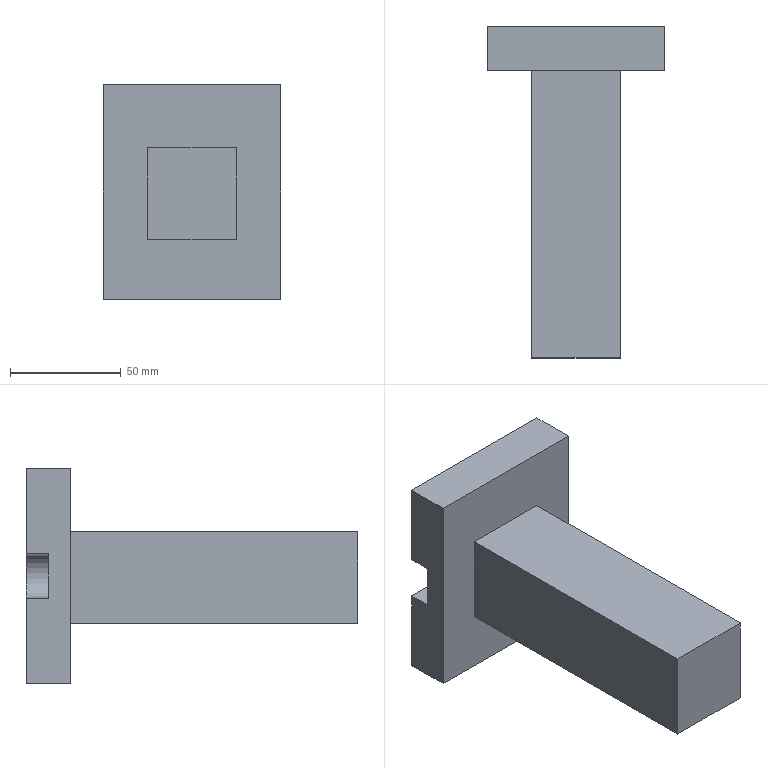Part | STEP file | Part1_4 | 1 solid | 15 faces | box 80 x 149.9 x 97 mm | volume 359263 mm3 | plane 14 | cylinder 1 | commonest cylinder face diameters 20 x1
STEP:
#1=CARTESIAN_POINT('',(0.,0.,0.));
#2=DIRECTION('',(0.,0.,1.));
#3=DIRECTION('',(1.,0.,0.));
#4=AXIS2_PLACEMENT_3D('',#1,#2,#3);
#5=CARTESIAN_POINT('',(10.,-29.9,-390.));
#6=VERTEX_POINT('',#5);
#7=CARTESIAN_POINT('',(-30.,-29.9,-390.));
#8=VERTEX_POINT('',#7);
#9=CARTESIAN_POINT('',(-30.,-29.9,-390.));
#10=DIRECTION('',(-1.,0.,0.));
#11=VECTOR('',#10,1.);
#12=LINE('',#9,#11);
#13=CARTESIAN_POINT('',(0.,-29.9,0.));
#14=DIRECTION('',(0.,1.,0.));
#15=DIRECTION('',(0.,0.,1.));
#16=AXIS2_PLACEMENT_3D('',#13,#14,#15);
#17=PLANE('',#16);
#18=CARTESIAN_POINT('',(-390.,-30.));
#19=DIRECTION('',(0.,-1.));
#20=VECTOR('',#19,1.);
#21=LINE('',#18,#20);
#22=(GEOMETRIC_REPRESENTATION_CONTEXT(2)PARAMETRIC_REPRESENTATION_CONTEXT()REPRESENTATION_CONTEXT('',''));
#23=DEFINITIONAL_REPRESENTATION('',(#21),#22);
#24=PCURVE('',#17,#23);
#25=CARTESIAN_POINT('',(-30.,100.,-390.));
#26=DIRECTION('',(0.,0.,-1.));
#27=DIRECTION('',(0.,1.,0.));
#28=AXIS2_PLACEMENT_3D('',#25,#26,#27);
#29=PLANE('',#28);
#30=CARTESIAN_POINT('',(-129.9,0.));
#31=DIRECTION('',(0.,-1.));
#32=VECTOR('',#31,1.);
#33=LINE('',#30,#32);
#34=(GEOMETRIC_REPRESENTATION_CONTEXT(2)PARAMETRIC_REPRESENTATION_CONTEXT()REPRESENTATION_CONTEXT('',''));
#35=DEFINITIONAL_REPRESENTATION('',(#33),#34);
#36=PCURVE('',#29,#35);
#37=SURFACE_CURVE('',#12,(#24,#36),.PCURVE_S1.);
#38=EDGE_CURVE('',#6,#8,#37,.T.);
#39=ORIENTED_EDGE('',*,*,#38,.T.);
#40=CARTESIAN_POINT('',(-30.,-29.9,-431.5));
#41=VERTEX_POINT('',#40);
#42=CARTESIAN_POINT('',(-30.,-29.9,-431.5));
#43=DIRECTION('',(0.,0.,-1.));
#44=VECTOR('',#43,1.);
#45=LINE('',#42,#44);
#46=CARTESIAN_POINT('',(-431.5,-30.));
#47=DIRECTION('',(-1.,0.));
#48=VECTOR('',#47,1.);
#49=LINE('',#46,#48);
#50=(GEOMETRIC_REPRESENTATION_CONTEXT(2)PARAMETRIC_REPRESENTATION_CONTEXT()REPRESENTATION_CONTEXT('',''));
#51=DEFINITIONAL_REPRESENTATION('',(#49),#50);
#52=PCURVE('',#17,#51);
#53=CARTESIAN_POINT('',(-30.,100.,-431.5));
#54=DIRECTION('',(1.,0.,0.));
#55=DIRECTION('',(0.,0.,-1.));
#56=AXIS2_PLACEMENT_3D('',#53,#54,#55);
#57=PLANE('',#56);
#58=CARTESIAN_POINT('',(0.,-129.9));
#59=DIRECTION('',(1.,0.));
#60=VECTOR('',#59,1.);
#61=LINE('',#58,#60);
#62=(GEOMETRIC_REPRESENTATION_CONTEXT(2)PARAMETRIC_REPRESENTATION_CONTEXT()REPRESENTATION_CONTEXT('',''));
#63=DEFINITIONAL_REPRESENTATION('',(#61),#62);
#64=PCURVE('',#57,#63);
#65=SURFACE_CURVE('',#45,(#52,#64),.PCURVE_S1.);
#66=EDGE_CURVE('',#8,#41,#65,.T.);
#67=ORIENTED_EDGE('',*,*,#66,.T.);
#68=CARTESIAN_POINT('',(10.,-29.9,-431.5));
#69=VERTEX_POINT('',#68);
#70=CARTESIAN_POINT('',(10.,-29.9,-431.5));
#71=DIRECTION('',(1.,0.,0.));
#72=VECTOR('',#71,1.);
#73=LINE('',#70,#72);
#74=CARTESIAN_POINT('',(-431.5,10.));
#75=DIRECTION('',(0.,1.));
#76=VECTOR('',#75,1.);
#77=LINE('',#74,#76);
#78=(GEOMETRIC_REPRESENTATION_CONTEXT(2)PARAMETRIC_REPRESENTATION_CONTEXT()REPRESENTATION_CONTEXT('',''));
#79=DEFINITIONAL_REPRESENTATION('',(#77),#78);
#80=PCURVE('',#17,#79);
#81=CARTESIAN_POINT('',(10.,100.,-431.5));
#82=DIRECTION('',(0.,0.,1.));
#83=DIRECTION('',(0.,-1.,0.));
#84=AXIS2_PLACEMENT_3D('',#81,#82,#83);
#85=PLANE('',#84);
#86=CARTESIAN_POINT('',(129.9,0.));
#87=DIRECTION('',(0.,1.));
#88=VECTOR('',#87,1.);
#89=LINE('',#86,#88);
#90=(GEOMETRIC_REPRESENTATION_CONTEXT(2)PARAMETRIC_REPRESENTATION_CONTEXT()REPRESENTATION_CONTEXT('',''));
#91=DEFINITIONAL_REPRESENTATION('',(#89),#90);
#92=PCURVE('',#85,#91);
#93=SURFACE_CURVE('',#73,(#80,#92),.PCURVE_S1.);
#94=EDGE_CURVE('',#41,#69,#93,.T.);
#95=ORIENTED_EDGE('',*,*,#94,.T.);
#96=CARTESIAN_POINT('',(10.,-29.9,-390.));
#97=DIRECTION('',(0.,0.,1.));
#98=VECTOR('',#97,1.);
#99=LINE('',#96,#98);
#100=CARTESIAN_POINT('',(-390.,10.));
#101=DIRECTION('',(1.,0.));
#102=VECTOR('',#101,1.);
#103=LINE('',#100,#102);
#104=(GEOMETRIC_REPRESENTATION_CONTEXT(2)PARAMETRIC_REPRESENTATION_CONTEXT()REPRESENTATION_CONTEXT('',''));
#105=DEFINITIONAL_REPRESENTATION('',(#103),#104);
#106=PCURVE('',#17,#105);
#107=CARTESIAN_POINT('',(10.,100.,-390.));
#108=DIRECTION('',(-1.,0.,0.));
#109=DIRECTION('',(0.,0.,1.));
#110=AXIS2_PLACEMENT_3D('',#107,#108,#109);
#111=PLANE('',#110);
#112=CARTESIAN_POINT('',(0.,-129.9));
#113=DIRECTION('',(1.,0.));
#114=VECTOR('',#113,1.);
#115=LINE('',#112,#114);
#116=(GEOMETRIC_REPRESENTATION_CONTEXT(2)PARAMETRIC_REPRESENTATION_CONTEXT()REPRESENTATION_CONTEXT('',''));
#117=DEFINITIONAL_REPRESENTATION('',(#115),#116);
#118=PCURVE('',#111,#117);
#119=SURFACE_CURVE('',#99,(#106,#118),.PCURVE_S1.);
#120=EDGE_CURVE('',#69,#6,#119,.T.);
#121=ORIENTED_EDGE('',*,*,#120,.T.);
#122=EDGE_LOOP('',(#39,#67,#95,#121));
#123=FACE_BOUND('',#122,.T.);
#124=ADVANCED_FACE('',(#123),#17,.F.);
#125=CARTESIAN_POINT('',(10.,100.,-431.5));
#126=VERTEX_POINT('',#125);
#127=CARTESIAN_POINT('',(10.,100.,-431.5));
#128=DIRECTION('',(0.,1.,0.));
#129=VECTOR('',#128,1.);
#130=LINE('',#127,#129);
#131=CARTESIAN_POINT('',(-41.5,0.));
#132=DIRECTION('',(0.,1.));
#133=VECTOR('',#132,1.);
#134=LINE('',#131,#133);
#135=(GEOMETRIC_REPRESENTATION_CONTEXT(2)PARAMETRIC_REPRESENTATION_CONTEXT()REPRESENTATION_CONTEXT('',''));
#136=DEFINITIONAL_REPRESENTATION('',(#134),#135);
#137=PCURVE('',#111,#136);
#138=CARTESIAN_POINT('',(0.,0.));
#139=DIRECTION('',(-1.,0.));
#140=VECTOR('',#139,1.);
#141=LINE('',#138,#140);
#142=(GEOMETRIC_REPRESENTATION_CONTEXT(2)PARAMETRIC_REPRESENTATION_CONTEXT()REPRESENTATION_CONTEXT('',''));
#143=DEFINITIONAL_REPRESENTATION('',(#141),#142);
#144=PCURVE('',#85,#143);
#145=SURFACE_CURVE('',#130,(#137,#144),.PCURVE_S1.);
#146=EDGE_CURVE('',#69,#126,#145,.T.);
#147=ORIENTED_EDGE('',*,*,#146,.T.);
#148=CARTESIAN_POINT('',(10.,100.,-390.));
#149=VERTEX_POINT('',#148);
#150=CARTESIAN_POINT('',(10.,100.,-361.5));
#151=DIRECTION('',(0.,0.,1.));
#152=VECTOR('',#151,1.);
#153=LINE('',#150,#152);
#154=CARTESIAN_POINT('',(28.5,0.));
#155=DIRECTION('',(1.,0.));
#156=VECTOR('',#155,1.);
#157=LINE('',#154,#156);
#158=(GEOMETRIC_REPRESENTATION_CONTEXT(2)PARAMETRIC_REPRESENTATION_CONTEXT()REPRESENTATION_CONTEXT('',''));
#159=DEFINITIONAL_REPRESENTATION('',(#157),#158);
#160=PCURVE('',#111,#159);
#161=CARTESIAN_POINT('',(-50.,100.,-361.5));
#162=DIRECTION('',(0.,1.,0.));
#163=DIRECTION('',(0.,0.,1.));
#164=AXIS2_PLACEMENT_3D('',#161,#162,#163);
#165=PLANE('',#164);
#166=CARTESIAN_POINT('',(0.,60.));
#167=DIRECTION('',(1.,0.));
#168=VECTOR('',#167,1.);
#169=LINE('',#166,#168);
#170=(GEOMETRIC_REPRESENTATION_CONTEXT(2)PARAMETRIC_REPRESENTATION_CONTEXT()REPRESENTATION_CONTEXT('',''));
#171=DEFINITIONAL_REPRESENTATION('',(#169),#170);
#172=PCURVE('',#165,#171);
#173=SURFACE_CURVE('',#153,(#160,#172),.PCURVE_S1.);
#174=EDGE_CURVE('',#126,#149,#173,.T.);
#175=ORIENTED_EDGE('',*,*,#174,.T.);
#176=CARTESIAN_POINT('',(10.,100.,-390.));
#177=DIRECTION('',(0.,-1.,0.));
#178=VECTOR('',#177,1.);
#179=LINE('',#176,#178);
#180=CARTESIAN_POINT('',(0.,0.));
#181=DIRECTION('',(0.,-1.));
#182=VECTOR('',#181,1.);
#183=LINE('',#180,#182);
#184=(GEOMETRIC_REPRESENTATION_CONTEXT(2)PARAMETRIC_REPRESENTATION_CONTEXT()REPRESENTATION_CONTEXT('',''));
#185=DEFINITIONAL_REPRESENTATION('',(#183),#184);
#186=PCURVE('',#111,#185);
#187=CARTESIAN_POINT('',(0.,40.));
#188=DIRECTION('',(-1.,0.));
#189=VECTOR('',#188,1.);
#190=LINE('',#187,#189);
#191=(GEOMETRIC_REPRESENTATION_CONTEXT(2)PARAMETRIC_REPRESENTATION_CONTEXT()REPRESENTATION_CONTEXT('',''));
#192=DEFINITIONAL_REPRESENTATION('',(#190),#191);
#193=PCURVE('',#29,#192);
#194=SURFACE_CURVE('',#179,(#186,#193),.PCURVE_S1.);
#195=EDGE_CURVE('',#149,#6,#194,.T.);
#196=ORIENTED_EDGE('',*,*,#195,.T.);
#197=ORIENTED_EDGE('',*,*,#120,.F.);
#198=EDGE_LOOP('',(#147,#175,#196,#197));
#199=FACE_BOUND('',#198,.T.);
#200=ADVANCED_FACE('',(#199),#111,.F.);
#201=ORIENTED_EDGE('',*,*,#195,.F.);
#202=CARTESIAN_POINT('',(-30.,100.,-390.));
#203=VERTEX_POINT('',#202);
#204=CARTESIAN_POINT('',(-50.,100.,-390.));
#205=DIRECTION('',(-1.,0.,0.));
#206=VECTOR('',#205,1.);
#207=LINE('',#204,#206);
#208=CARTESIAN_POINT('',(0.,-20.));
#209=DIRECTION('',(0.,-1.));
#210=VECTOR('',#209,1.);
#211=LINE('',#208,#210);
#212=(GEOMETRIC_REPRESENTATION_CONTEXT(2)PARAMETRIC_REPRESENTATION_CONTEXT()REPRESENTATION_CONTEXT('',''));
#213=DEFINITIONAL_REPRESENTATION('',(#211),#212);
#214=PCURVE('',#29,#213);
#215=CARTESIAN_POINT('',(-28.5,0.));
#216=DIRECTION('',(0.,-1.));
#217=VECTOR('',#216,1.);
#218=LINE('',#215,#217);
#219=(GEOMETRIC_REPRESENTATION_CONTEXT(2)PARAMETRIC_REPRESENTATION_CONTEXT()REPRESENTATION_CONTEXT('',''));
#220=DEFINITIONAL_REPRESENTATION('',(#218),#219);
#221=PCURVE('',#165,#220);
#222=SURFACE_CURVE('',#207,(#214,#221),.PCURVE_S1.);
#223=EDGE_CURVE('',#149,#203,#222,.T.);
#224=ORIENTED_EDGE('',*,*,#223,.T.);
#225=CARTESIAN_POINT('',(-30.,100.,-390.));
#226=DIRECTION('',(0.,-1.,0.));
#227=VECTOR('',#226,1.);
#228=LINE('',#225,#227);
#229=CARTESIAN_POINT('',(0.,0.));
#230=DIRECTION('',(-1.,0.));
#231=VECTOR('',#230,1.);
#232=LINE('',#229,#231);
#233=(GEOMETRIC_REPRESENTATION_CONTEXT(2)PARAMETRIC_REPRESENTATION_CONTEXT()REPRESENTATION_CONTEXT('',''));
#234=DEFINITIONAL_REPRESENTATION('',(#232),#233);
#235=PCURVE('',#29,#234);
#236=CARTESIAN_POINT('',(-41.5,0.));
#237=DIRECTION('',(0.,-1.));
#238=VECTOR('',#237,1.);
#239=LINE('',#236,#238);
#240=(GEOMETRIC_REPRESENTATION_CONTEXT(2)PARAMETRIC_REPRESENTATION_CONTEXT()REPRESENTATION_CONTEXT('',''));
#241=DEFINITIONAL_REPRESENTATION('',(#239),#240);
#242=PCURVE('',#57,#241);
#243=SURFACE_CURVE('',#228,(#235,#242),.PCURVE_S1.);
#244=EDGE_CURVE('',#203,#8,#243,.T.);
#245=ORIENTED_EDGE('',*,*,#244,.T.);
#246=ORIENTED_EDGE('',*,*,#38,.F.);
#247=EDGE_LOOP('',(#201,#224,#245,#246));
#248=FACE_BOUND('',#247,.T.);
#249=ADVANCED_FACE('',(#248),#29,.F.);
#250=ORIENTED_EDGE('',*,*,#244,.F.);
#251=CARTESIAN_POINT('',(-30.,100.,-431.5));
#252=VERTEX_POINT('',#251);
#253=CARTESIAN_POINT('',(-30.,100.,-361.5));
#254=DIRECTION('',(0.,0.,-1.));
#255=VECTOR('',#254,1.);
#256=LINE('',#253,#255);
#257=CARTESIAN_POINT('',(-70.,0.));
#258=DIRECTION('',(1.,0.));
#259=VECTOR('',#258,1.);
#260=LINE('',#257,#259);
#261=(GEOMETRIC_REPRESENTATION_CONTEXT(2)PARAMETRIC_REPRESENTATION_CONTEXT()REPRESENTATION_CONTEXT('',''));
#262=DEFINITIONAL_REPRESENTATION('',(#260),#261);
#263=PCURVE('',#57,#262);
#264=CARTESIAN_POINT('',(0.,20.));
#265=DIRECTION('',(-1.,0.));
#266=VECTOR('',#265,1.);
#267=LINE('',#264,#266);
#268=(GEOMETRIC_REPRESENTATION_CONTEXT(2)PARAMETRIC_REPRESENTATION_CONTEXT()REPRESENTATION_CONTEXT('',''));
#269=DEFINITIONAL_REPRESENTATION('',(#267),#268);
#270=PCURVE('',#165,#269);
#271=SURFACE_CURVE('',#256,(#263,#270),.PCURVE_S1.);
#272=EDGE_CURVE('',#203,#252,#271,.T.);
#273=ORIENTED_EDGE('',*,*,#272,.T.);
#274=CARTESIAN_POINT('',(-30.,100.,-431.5));
#275=DIRECTION('',(0.,-1.,0.));
#276=VECTOR('',#275,1.);
#277=LINE('',#274,#276);
#278=CARTESIAN_POINT('',(0.,0.));
#279=DIRECTION('',(0.,-1.));
#280=VECTOR('',#279,1.);
#281=LINE('',#278,#280);
#282=(GEOMETRIC_REPRESENTATION_CONTEXT(2)PARAMETRIC_REPRESENTATION_CONTEXT()REPRESENTATION_CONTEXT('',''));
#283=DEFINITIONAL_REPRESENTATION('',(#281),#282);
#284=PCURVE('',#57,#283);
#285=CARTESIAN_POINT('',(0.,-40.));
#286=DIRECTION('',(1.,0.));
#287=VECTOR('',#286,1.);
#288=LINE('',#285,#287);
#289=(GEOMETRIC_REPRESENTATION_CONTEXT(2)PARAMETRIC_REPRESENTATION_CONTEXT()REPRESENTATION_CONTEXT('',''));
#290=DEFINITIONAL_REPRESENTATION('',(#288),#289);
#291=PCURVE('',#85,#290);
#292=SURFACE_CURVE('',#277,(#284,#291),.PCURVE_S1.);
#293=EDGE_CURVE('',#252,#41,#292,.T.);
#294=ORIENTED_EDGE('',*,*,#293,.T.);
#295=ORIENTED_EDGE('',*,*,#66,.F.);
#296=EDGE_LOOP('',(#250,#273,#294,#295));
#297=FACE_BOUND('',#296,.T.);
#298=ADVANCED_FACE('',(#297),#57,.F.);
#299=ORIENTED_EDGE('',*,*,#293,.F.);
#300=CARTESIAN_POINT('',(-50.,100.,-431.5));
#301=DIRECTION('',(1.,0.,0.));
#302=VECTOR('',#301,1.);
#303=LINE('',#300,#302);
#304=CARTESIAN_POINT('',(0.,-60.));
#305=DIRECTION('',(0.,1.));
#306=VECTOR('',#305,1.);
#307=LINE('',#304,#306);
#308=(GEOMETRIC_REPRESENTATION_CONTEXT(2)PARAMETRIC_REPRESENTATION_CONTEXT()REPRESENTATION_CONTEXT('',''));
#309=DEFINITIONAL_REPRESENTATION('',(#307),#308);
#310=PCURVE('',#85,#309);
#311=CARTESIAN_POINT('',(-70.,0.));
#312=DIRECTION('',(0.,1.));
#313=VECTOR('',#312,1.);
#314=LINE('',#311,#313);
#315=(GEOMETRIC_REPRESENTATION_CONTEXT(2)PARAMETRIC_REPRESENTATION_CONTEXT()REPRESENTATION_CONTEXT('',''));
#316=DEFINITIONAL_REPRESENTATION('',(#314),#315);
#317=PCURVE('',#165,#316);
#318=SURFACE_CURVE('',#303,(#310,#317),.PCURVE_S1.);
#319=EDGE_CURVE('',#252,#126,#318,.T.);
#320=ORIENTED_EDGE('',*,*,#319,.T.);
#321=ORIENTED_EDGE('',*,*,#146,.F.);
#322=ORIENTED_EDGE('',*,*,#94,.F.);
#323=EDGE_LOOP('',(#299,#320,#321,#322));
#324=FACE_BOUND('',#323,.T.);
#325=ADVANCED_FACE('',(#324),#85,.F.);
#326=ORIENTED_EDGE('',*,*,#272,.F.);
#327=ORIENTED_EDGE('',*,*,#223,.F.);
#328=ORIENTED_EDGE('',*,*,#174,.F.);
#329=ORIENTED_EDGE('',*,*,#319,.F.);
#330=EDGE_LOOP('',(#326,#327,#328,#329));
#331=FACE_BOUND('',#330,.T.);
#332=CARTESIAN_POINT('',(30.,100.,-361.5));
#333=VERTEX_POINT('',#332);
#334=CARTESIAN_POINT('',(30.,100.,-458.5));
#335=VERTEX_POINT('',#334);
#336=CARTESIAN_POINT('',(30.,100.,-361.5));
#337=DIRECTION('',(0.,0.,-1.));
#338=VECTOR('',#337,1.);
#339=LINE('',#336,#338);
#340=CARTESIAN_POINT('',(0.,80.));
#341=DIRECTION('',(-1.,0.));
#342=VECTOR('',#341,1.);
#343=LINE('',#340,#342);
#344=(GEOMETRIC_REPRESENTATION_CONTEXT(2)PARAMETRIC_REPRESENTATION_CONTEXT()REPRESENTATION_CONTEXT('',''));
#345=DEFINITIONAL_REPRESENTATION('',(#343),#344);
#346=PCURVE('',#165,#345);
#347=CARTESIAN_POINT('',(30.,120.,-361.5));
#348=DIRECTION('',(1.,0.,0.));
#349=DIRECTION('',(0.,0.,-1.));
#350=AXIS2_PLACEMENT_3D('',#347,#348,#349);
#351=PLANE('',#350);
#352=CARTESIAN_POINT('',(0.,-20.));
#353=DIRECTION('',(1.,0.));
#354=VECTOR('',#353,1.);
#355=LINE('',#352,#354);
#356=(GEOMETRIC_REPRESENTATION_CONTEXT(2)PARAMETRIC_REPRESENTATION_CONTEXT()REPRESENTATION_CONTEXT('',''));
#357=DEFINITIONAL_REPRESENTATION('',(#355),#356);
#358=PCURVE('',#351,#357);
#359=SURFACE_CURVE('',#339,(#346,#358),.PCURVE_S1.);
#360=EDGE_CURVE('',#333,#335,#359,.T.);
#361=ORIENTED_EDGE('',*,*,#360,.F.);
#362=CARTESIAN_POINT('',(-50.,100.,-361.5));
#363=VERTEX_POINT('',#362);
#364=CARTESIAN_POINT('',(0.,100.,-361.5));
#365=DIRECTION('',(1.,0.,0.));
#366=VECTOR('',#365,1.);
#367=LINE('',#364,#366);
#368=CARTESIAN_POINT('',(0.,50.));
#369=DIRECTION('',(0.,1.));
#370=VECTOR('',#369,1.);
#371=LINE('',#368,#370);
#372=(GEOMETRIC_REPRESENTATION_CONTEXT(2)PARAMETRIC_REPRESENTATION_CONTEXT()REPRESENTATION_CONTEXT('',''));
#373=DEFINITIONAL_REPRESENTATION('',(#371),#372);
#374=PCURVE('',#165,#373);
#375=CARTESIAN_POINT('',(0.,0.,-361.5));
#376=DIRECTION('',(0.,0.,1.));
#377=DIRECTION('',(1.,0.,0.));
#378=AXIS2_PLACEMENT_3D('',#375,#376,#377);
#379=PLANE('',#378);
#380=CARTESIAN_POINT('',(0.,100.));
#381=DIRECTION('',(1.,0.));
#382=VECTOR('',#381,1.);
#383=LINE('',#380,#382);
#384=(GEOMETRIC_REPRESENTATION_CONTEXT(2)PARAMETRIC_REPRESENTATION_CONTEXT()REPRESENTATION_CONTEXT('',''));
#385=DEFINITIONAL_REPRESENTATION('',(#383),#384);
#386=PCURVE('',#379,#385);
#387=SURFACE_CURVE('',#367,(#374,#386),.PCURVE_S1.);
#388=EDGE_CURVE('',#363,#333,#387,.T.);
#389=ORIENTED_EDGE('',*,*,#388,.F.);
#390=CARTESIAN_POINT('',(-50.,100.,-458.5));
#391=VERTEX_POINT('',#390);
#392=CARTESIAN_POINT('',(-50.,100.,-361.5));
#393=DIRECTION('',(0.,0.,1.));
#394=VECTOR('',#393,1.);
#395=LINE('',#392,#394);
#396=CARTESIAN_POINT('',(0.,0.));
#397=DIRECTION('',(1.,0.));
#398=VECTOR('',#397,1.);
#399=LINE('',#396,#398);
#400=(GEOMETRIC_REPRESENTATION_CONTEXT(2)PARAMETRIC_REPRESENTATION_CONTEXT()REPRESENTATION_CONTEXT('',''));
#401=DEFINITIONAL_REPRESENTATION('',(#399),#400);
#402=PCURVE('',#165,#401);
#403=CARTESIAN_POINT('',(-50.,100.,-361.5));
#404=DIRECTION('',(-1.,0.,0.));
#405=DIRECTION('',(0.,0.,1.));
#406=AXIS2_PLACEMENT_3D('',#403,#404,#405);
#407=PLANE('',#406);
#408=CARTESIAN_POINT('',(0.,0.));
#409=DIRECTION('',(1.,0.));
#410=VECTOR('',#409,1.);
#411=LINE('',#408,#410);
#412=(GEOMETRIC_REPRESENTATION_CONTEXT(2)PARAMETRIC_REPRESENTATION_CONTEXT()REPRESENTATION_CONTEXT('',''));
#413=DEFINITIONAL_REPRESENTATION('',(#411),#412);
#414=PCURVE('',#407,#413);
#415=SURFACE_CURVE('',#395,(#402,#414),.PCURVE_S1.);
#416=EDGE_CURVE('',#391,#363,#415,.T.);
#417=ORIENTED_EDGE('',*,*,#416,.F.);
#418=CARTESIAN_POINT('',(-25.,100.,-458.5));
#419=DIRECTION('',(-1.,0.,0.));
#420=VECTOR('',#419,1.);
#421=LINE('',#418,#420);
#422=CARTESIAN_POINT('',(-97.,25.));
#423=DIRECTION('',(0.,-1.));
#424=VECTOR('',#423,1.);
#425=LINE('',#422,#424);
#426=(GEOMETRIC_REPRESENTATION_CONTEXT(2)PARAMETRIC_REPRESENTATION_CONTEXT()REPRESENTATION_CONTEXT('',''));
#427=DEFINITIONAL_REPRESENTATION('',(#425),#426);
#428=PCURVE('',#165,#427);
#429=CARTESIAN_POINT('',(-25.,377.,-458.5));
#430=DIRECTION('',(0.,0.,-1.));
#431=DIRECTION('',(-1.,0.,0.));
#432=AXIS2_PLACEMENT_3D('',#429,#430,#431);
#433=PLANE('',#432);
#434=CARTESIAN_POINT('',(0.,-277.));
#435=DIRECTION('',(1.,0.));
#436=VECTOR('',#435,1.);
#437=LINE('',#434,#436);
#438=(GEOMETRIC_REPRESENTATION_CONTEXT(2)PARAMETRIC_REPRESENTATION_CONTEXT()REPRESENTATION_CONTEXT('',''));
#439=DEFINITIONAL_REPRESENTATION('',(#437),#438);
#440=PCURVE('',#433,#439);
#441=SURFACE_CURVE('',#421,(#428,#440),.PCURVE_S1.);
#442=EDGE_CURVE('',#335,#391,#441,.T.);
#443=ORIENTED_EDGE('',*,*,#442,.F.);
#444=EDGE_LOOP('',(#361,#389,#417,#443));
#445=FACE_BOUND('',#444,.T.);
#446=ADVANCED_FACE('',(#331,#445),#165,.F.);
#447=CARTESIAN_POINT('',(0.,110.,-420.));
#448=VERTEX_POINT('',#447);
#449=CARTESIAN_POINT('',(-50.,110.,-420.));
#450=VERTEX_POINT('',#449);
#451=CARTESIAN_POINT('',(-60.,110.,-420.));
#452=DIRECTION('',(-1.,0.,0.));
#453=VECTOR('',#452,1.);
#454=LINE('',#451,#453);
#455=CARTESIAN_POINT('',(0.,110.,0.));
#456=DIRECTION('',(0.,1.,0.));
#457=DIRECTION('',(0.,0.,1.));
#458=AXIS2_PLACEMENT_3D('',#455,#456,#457);
#459=PLANE('',#458);
#460=CARTESIAN_POINT('',(-420.,-60.));
#461=DIRECTION('',(0.,-1.));
#462=VECTOR('',#461,1.);
#463=LINE('',#460,#462);
#464=(GEOMETRIC_REPRESENTATION_CONTEXT(2)PARAMETRIC_REPRESENTATION_CONTEXT()REPRESENTATION_CONTEXT('',''));
#465=DEFINITIONAL_REPRESENTATION('',(#463),#464);
#466=PCURVE('',#459,#465);
#467=CARTESIAN_POINT('',(-60.,120.,-420.));
#468=DIRECTION('',(0.,0.,-1.));
#469=DIRECTION('',(0.,1.,0.));
#470=AXIS2_PLACEMENT_3D('',#467,#468,#469);
#471=PLANE('',#470);
#472=CARTESIAN_POINT('',(-10.,0.));
#473=DIRECTION('',(0.,-1.));
#474=VECTOR('',#473,1.);
#475=LINE('',#472,#474);
#476=(GEOMETRIC_REPRESENTATION_CONTEXT(2)PARAMETRIC_REPRESENTATION_CONTEXT()REPRESENTATION_CONTEXT('',''));
#477=DEFINITIONAL_REPRESENTATION('',(#475),#476);
#478=PCURVE('',#471,#477);
#479=SURFACE_CURVE('',#454,(#466,#478),.PCURVE_S1.);
#480=EDGE_CURVE('',#448,#450,#479,.T.);
#481=ORIENTED_EDGE('',*,*,#480,.T.);
#482=CARTESIAN_POINT('',(-50.,110.,-400.));
#483=VERTEX_POINT('',#482);
#484=CARTESIAN_POINT('',(-50.,110.,-361.5));
#485=DIRECTION('',(0.,0.,-1.));
#486=VECTOR('',#485,1.);
#487=LINE('',#484,#486);
#488=CARTESIAN_POINT('',(-361.5,-50.));
#489=DIRECTION('',(-1.,0.));
#490=VECTOR('',#489,1.);
#491=LINE('',#488,#490);
#492=(GEOMETRIC_REPRESENTATION_CONTEXT(2)PARAMETRIC_REPRESENTATION_CONTEXT()REPRESENTATION_CONTEXT('',''));
#493=DEFINITIONAL_REPRESENTATION('',(#491),#492);
#494=PCURVE('',#459,#493);
#495=CARTESIAN_POINT('',(0.,10.));
#496=DIRECTION('',(-1.,0.));
#497=VECTOR('',#496,1.);
#498=LINE('',#495,#497);
#499=(GEOMETRIC_REPRESENTATION_CONTEXT(2)PARAMETRIC_REPRESENTATION_CONTEXT()REPRESENTATION_CONTEXT('',''));
#500=DEFINITIONAL_REPRESENTATION('',(#498),#499);
#501=PCURVE('',#407,#500);
#502=SURFACE_CURVE('',#487,(#494,#501),.PCURVE_S1.);
#503=EDGE_CURVE('',#483,#450,#502,.T.);
#504=ORIENTED_EDGE('',*,*,#503,.F.);
#505=CARTESIAN_POINT('',(0.,110.,-400.));
#506=VERTEX_POINT('',#505);
#507=CARTESIAN_POINT('',(0.,110.,-400.));
#508=DIRECTION('',(1.,0.,0.));
#509=VECTOR('',#508,1.);
#510=LINE('',#507,#509);
#511=CARTESIAN_POINT('',(-400.,0.));
#512=DIRECTION('',(0.,1.));
#513=VECTOR('',#512,1.);
#514=LINE('',#511,#513);
#515=(GEOMETRIC_REPRESENTATION_CONTEXT(2)PARAMETRIC_REPRESENTATION_CONTEXT()REPRESENTATION_CONTEXT('',''));
#516=DEFINITIONAL_REPRESENTATION('',(#514),#515);
#517=PCURVE('',#459,#516);
#518=CARTESIAN_POINT('',(0.,120.,-400.));
#519=DIRECTION('',(0.,0.,1.));
#520=DIRECTION('',(0.,-1.,0.));
#521=AXIS2_PLACEMENT_3D('',#518,#519,#520);
#522=PLANE('',#521);
#523=CARTESIAN_POINT('',(10.,0.));
#524=DIRECTION('',(0.,1.));
#525=VECTOR('',#524,1.);
#526=LINE('',#523,#525);
#527=(GEOMETRIC_REPRESENTATION_CONTEXT(2)PARAMETRIC_REPRESENTATION_CONTEXT()REPRESENTATION_CONTEXT('',''));
#528=DEFINITIONAL_REPRESENTATION('',(#526),#527);
#529=PCURVE('',#522,#528);
#530=SURFACE_CURVE('',#510,(#517,#529),.PCURVE_S1.);
#531=EDGE_CURVE('',#483,#506,#530,.T.);
#532=ORIENTED_EDGE('',*,*,#531,.T.);
#533=CARTESIAN_POINT('',(0.,110.,-410.));
#534=DIRECTION('',(0.,1.,0.));
#535=DIRECTION('',(0.,0.,1.));
#536=AXIS2_PLACEMENT_3D('',#533,#534,#535);
#537=CIRCLE('',#536,10.);
#538=CARTESIAN_POINT('',(-410.,0.));
#539=DIRECTION('',(1.,0.));
#540=AXIS2_PLACEMENT_2D('',#538,#539);
#541=CIRCLE('',#540,10.);
#542=(GEOMETRIC_REPRESENTATION_CONTEXT(2)PARAMETRIC_REPRESENTATION_CONTEXT()REPRESENTATION_CONTEXT('',''));
#543=DEFINITIONAL_REPRESENTATION('',(#541),#542);
#544=PCURVE('',#459,#543);
#545=CARTESIAN_POINT('',(0.,115.,-410.));
#546=DIRECTION('',(0.,1.,0.));
#547=DIRECTION('',(0.,0.,1.));
#548=AXIS2_PLACEMENT_3D('',#545,#546,#547);
#549=CYLINDRICAL_SURFACE('',#548,10.);
#550=CARTESIAN_POINT('',(0.,-5.));
#551=DIRECTION('',(1.,0.));
#552=VECTOR('',#551,1.);
#553=LINE('',#550,#552);
#554=(GEOMETRIC_REPRESENTATION_CONTEXT(2)PARAMETRIC_REPRESENTATION_CONTEXT()REPRESENTATION_CONTEXT('',''));
#555=DEFINITIONAL_REPRESENTATION('',(#553),#554);
#556=PCURVE('',#549,#555);
#557=SURFACE_CURVE('',#537,(#544,#556),.PCURVE_S1.);
#558=EDGE_CURVE('',#506,#448,#557,.T.);
#559=ORIENTED_EDGE('',*,*,#558,.T.);
#560=EDGE_LOOP('',(#481,#504,#532,#559));
#561=FACE_BOUND('',#560,.T.);
#562=ADVANCED_FACE('',(#561),#459,.T.);
#563=CARTESIAN_POINT('',(30.,120.,-458.5));
#564=VERTEX_POINT('',#563);
#565=CARTESIAN_POINT('',(30.,120.,-458.5));
#566=DIRECTION('',(0.,1.,0.));
#567=VECTOR('',#566,1.);
#568=LINE('',#565,#567);
#569=CARTESIAN_POINT('',(-55.,-257.));
#570=DIRECTION('',(0.,1.));
#571=VECTOR('',#570,1.);
#572=LINE('',#569,#571);
#573=(GEOMETRIC_REPRESENTATION_CONTEXT(2)PARAMETRIC_REPRESENTATION_CONTEXT()REPRESENTATION_CONTEXT('',''));
#574=DEFINITIONAL_REPRESENTATION('',(#572),#573);
#575=PCURVE('',#433,#574);
#576=CARTESIAN_POINT('',(97.,0.));
#577=DIRECTION('',(0.,1.));
#578=VECTOR('',#577,1.);
#579=LINE('',#576,#578);
#580=(GEOMETRIC_REPRESENTATION_CONTEXT(2)PARAMETRIC_REPRESENTATION_CONTEXT()REPRESENTATION_CONTEXT('',''));
#581=DEFINITIONAL_REPRESENTATION('',(#579),#580);
#582=PCURVE('',#351,#581);
#583=SURFACE_CURVE('',#568,(#575,#582),.PCURVE_S1.);
#584=EDGE_CURVE('',#335,#564,#583,.T.);
#585=ORIENTED_EDGE('',*,*,#584,.F.);
#586=ORIENTED_EDGE('',*,*,#442,.T.);
#587=CARTESIAN_POINT('',(-50.,120.,-458.5));
#588=VERTEX_POINT('',#587);
#589=CARTESIAN_POINT('',(-50.,100.,-458.5));
#590=DIRECTION('',(0.,-1.,0.));
#591=VECTOR('',#590,1.);
#592=LINE('',#589,#591);
#593=CARTESIAN_POINT('',(25.,-277.));
#594=DIRECTION('',(0.,-1.));
#595=VECTOR('',#594,1.);
#596=LINE('',#593,#595);
#597=(GEOMETRIC_REPRESENTATION_CONTEXT(2)PARAMETRIC_REPRESENTATION_CONTEXT()REPRESENTATION_CONTEXT('',''));
#598=DEFINITIONAL_REPRESENTATION('',(#596),#597);
#599=PCURVE('',#433,#598);
#600=CARTESIAN_POINT('',(-97.,0.));
#601=DIRECTION('',(0.,-1.));
#602=VECTOR('',#601,1.);
#603=LINE('',#600,#602);
#604=(GEOMETRIC_REPRESENTATION_CONTEXT(2)PARAMETRIC_REPRESENTATION_CONTEXT()REPRESENTATION_CONTEXT('',''));
#605=DEFINITIONAL_REPRESENTATION('',(#603),#604);
#606=PCURVE('',#407,#605);
#607=SURFACE_CURVE('',#592,(#599,#606),.PCURVE_S1.);
#608=EDGE_CURVE('',#588,#391,#607,.T.);
#609=ORIENTED_EDGE('',*,*,#608,.F.);
#610=CARTESIAN_POINT('',(30.,120.,-458.5));
#611=DIRECTION('',(1.,0.,0.));
#612=VECTOR('',#611,1.);
#613=LINE('',#610,#612);
#614=CARTESIAN_POINT('',(-55.,-257.));
#615=DIRECTION('',(-1.,0.));
#616=VECTOR('',#615,1.);
#617=LINE('',#614,#616);
#618=(GEOMETRIC_REPRESENTATION_CONTEXT(2)PARAMETRIC_REPRESENTATION_CONTEXT()REPRESENTATION_CONTEXT('',''));
#619=DEFINITIONAL_REPRESENTATION('',(#617),#618);
#620=PCURVE('',#433,#619);
#621=CARTESIAN_POINT('',(30.,120.,-361.5));
#622=DIRECTION('',(0.,-1.,0.));
#623=DIRECTION('',(0.,0.,-1.));
#624=AXIS2_PLACEMENT_3D('',#621,#622,#623);
#625=PLANE('',#624);
#626=CARTESIAN_POINT('',(97.,0.));
#627=DIRECTION('',(0.,1.));
#628=VECTOR('',#627,1.);
#629=LINE('',#626,#628);
#630=(GEOMETRIC_REPRESENTATION_CONTEXT(2)PARAMETRIC_REPRESENTATION_CONTEXT()REPRESENTATION_CONTEXT('',''));
#631=DEFINITIONAL_REPRESENTATION('',(#629),#630);
#632=PCURVE('',#625,#631);
#633=SURFACE_CURVE('',#613,(#620,#632),.PCURVE_S1.);
#634=EDGE_CURVE('',#588,#564,#633,.T.);
#635=ORIENTED_EDGE('',*,*,#634,.T.);
#636=EDGE_LOOP('',(#585,#586,#609,#635));
#637=FACE_BOUND('',#636,.T.);
#638=ADVANCED_FACE('',(#637),#433,.T.);
#639=ORIENTED_EDGE('',*,*,#360,.T.);
#640=ORIENTED_EDGE('',*,*,#584,.T.);
#641=CARTESIAN_POINT('',(30.,120.,-361.5));
#642=VERTEX_POINT('',#641);
#643=CARTESIAN_POINT('',(30.,120.,-361.5));
#644=DIRECTION('',(0.,0.,1.));
#645=VECTOR('',#644,1.);
#646=LINE('',#643,#645);
#647=CARTESIAN_POINT('',(0.,0.));
#648=DIRECTION('',(-1.,0.));
#649=VECTOR('',#648,1.);
#650=LINE('',#647,#649);
#651=(GEOMETRIC_REPRESENTATION_CONTEXT(2)PARAMETRIC_REPRESENTATION_CONTEXT()REPRESENTATION_CONTEXT('',''));
#652=DEFINITIONAL_REPRESENTATION('',(#650),#651);
#653=PCURVE('',#351,#652);
#654=CARTESIAN_POINT('',(0.,0.));
#655=DIRECTION('',(-1.,0.));
#656=VECTOR('',#655,1.);
#657=LINE('',#654,#656);
#658=(GEOMETRIC_REPRESENTATION_CONTEXT(2)PARAMETRIC_REPRESENTATION_CONTEXT()REPRESENTATION_CONTEXT('',''));
#659=DEFINITIONAL_REPRESENTATION('',(#657),#658);
#660=PCURVE('',#625,#659);
#661=SURFACE_CURVE('',#646,(#653,#660),.PCURVE_S1.);
#662=EDGE_CURVE('',#564,#642,#661,.T.);
#663=ORIENTED_EDGE('',*,*,#662,.T.);
#664=CARTESIAN_POINT('',(30.,0.,-361.5));
#665=DIRECTION('',(0.,1.,0.));
#666=VECTOR('',#665,1.);
#667=LINE('',#664,#666);
#668=CARTESIAN_POINT('',(0.,-120.));
#669=DIRECTION('',(0.,1.));
#670=VECTOR('',#669,1.);
#671=LINE('',#668,#670);
#672=(GEOMETRIC_REPRESENTATION_CONTEXT(2)PARAMETRIC_REPRESENTATION_CONTEXT()REPRESENTATION_CONTEXT('',''));
#673=DEFINITIONAL_REPRESENTATION('',(#671),#672);
#674=PCURVE('',#351,#673);
#675=CARTESIAN_POINT('',(30.,0.));
#676=DIRECTION('',(0.,1.));
#677=VECTOR('',#676,1.);
#678=LINE('',#675,#677);
#679=(GEOMETRIC_REPRESENTATION_CONTEXT(2)PARAMETRIC_REPRESENTATION_CONTEXT()REPRESENTATION_CONTEXT('',''));
#680=DEFINITIONAL_REPRESENTATION('',(#678),#679);
#681=PCURVE('',#379,#680);
#682=SURFACE_CURVE('',#667,(#674,#681),.PCURVE_S1.);
#683=EDGE_CURVE('',#333,#642,#682,.T.);
#684=ORIENTED_EDGE('',*,*,#683,.F.);
#685=EDGE_LOOP('',(#639,#640,#663,#684));
#686=FACE_BOUND('',#685,.T.);
#687=ADVANCED_FACE('',(#686),#351,.T.);
#688=CARTESIAN_POINT('',(-50.,120.,-361.5));
#689=VERTEX_POINT('',#688);
#690=CARTESIAN_POINT('',(-50.,100.,-361.5));
#691=DIRECTION('',(0.,1.,0.));
#692=VECTOR('',#691,1.);
#693=LINE('',#690,#692);
#694=CARTESIAN_POINT('',(-50.,100.));
#695=DIRECTION('',(0.,1.));
#696=VECTOR('',#695,1.);
#697=LINE('',#694,#696);
#698=(GEOMETRIC_REPRESENTATION_CONTEXT(2)PARAMETRIC_REPRESENTATION_CONTEXT()REPRESENTATION_CONTEXT('',''));
#699=DEFINITIONAL_REPRESENTATION('',(#697),#698);
#700=PCURVE('',#379,#699);
#701=CARTESIAN_POINT('',(0.,0.));
#702=DIRECTION('',(0.,1.));
#703=VECTOR('',#702,1.);
#704=LINE('',#701,#703);
#705=(GEOMETRIC_REPRESENTATION_CONTEXT(2)PARAMETRIC_REPRESENTATION_CONTEXT()REPRESENTATION_CONTEXT('',''));
#706=DEFINITIONAL_REPRESENTATION('',(#704),#705);
#707=PCURVE('',#407,#706);
#708=SURFACE_CURVE('',#693,(#700,#707),.PCURVE_S1.);
#709=EDGE_CURVE('',#363,#689,#708,.T.);
#710=ORIENTED_EDGE('',*,*,#709,.F.);
#711=ORIENTED_EDGE('',*,*,#388,.T.);
#712=ORIENTED_EDGE('',*,*,#683,.T.);
#713=CARTESIAN_POINT('',(30.,120.,-361.5));
#714=DIRECTION('',(-1.,0.,0.));
#715=VECTOR('',#714,1.);
#716=LINE('',#713,#715);
#717=CARTESIAN_POINT('',(30.,120.));
#718=DIRECTION('',(-1.,0.));
#719=VECTOR('',#718,1.);
#720=LINE('',#717,#719);
#721=(GEOMETRIC_REPRESENTATION_CONTEXT(2)PARAMETRIC_REPRESENTATION_CONTEXT()REPRESENTATION_CONTEXT('',''));
#722=DEFINITIONAL_REPRESENTATION('',(#720),#721);
#723=PCURVE('',#379,#722);
#724=CARTESIAN_POINT('',(0.,0.));
#725=DIRECTION('',(0.,-1.));
#726=VECTOR('',#725,1.);
#727=LINE('',#724,#726);
#728=(GEOMETRIC_REPRESENTATION_CONTEXT(2)PARAMETRIC_REPRESENTATION_CONTEXT()REPRESENTATION_CONTEXT('',''));
#729=DEFINITIONAL_REPRESENTATION('',(#727),#728);
#730=PCURVE('',#625,#729);
#731=SURFACE_CURVE('',#716,(#723,#730),.PCURVE_S1.);
#732=EDGE_CURVE('',#642,#689,#731,.T.);
#733=ORIENTED_EDGE('',*,*,#732,.T.);
#734=EDGE_LOOP('',(#710,#711,#712,#733));
#735=FACE_BOUND('',#734,.T.);
#736=ADVANCED_FACE('',(#735),#379,.T.);
#737=ORIENTED_EDGE('',*,*,#503,.T.);
#738=CARTESIAN_POINT('',(-50.,120.,-420.));
#739=VERTEX_POINT('',#738);
#740=CARTESIAN_POINT('',(-50.,120.,-420.));
#741=DIRECTION('',(0.,1.,0.));
#742=VECTOR('',#741,1.);
#743=LINE('',#740,#742);
#744=CARTESIAN_POINT('',(-58.5,20.));
#745=DIRECTION('',(0.,1.));
#746=VECTOR('',#745,1.);
#747=LINE('',#744,#746);
#748=(GEOMETRIC_REPRESENTATION_CONTEXT(2)PARAMETRIC_REPRESENTATION_CONTEXT()REPRESENTATION_CONTEXT('',''));
#749=DEFINITIONAL_REPRESENTATION('',(#747),#748);
#750=PCURVE('',#407,#749);
#751=CARTESIAN_POINT('',(0.,10.));
#752=DIRECTION('',(1.,0.));
#753=VECTOR('',#752,1.);
#754=LINE('',#751,#753);
#755=(GEOMETRIC_REPRESENTATION_CONTEXT(2)PARAMETRIC_REPRESENTATION_CONTEXT()REPRESENTATION_CONTEXT('',''));
#756=DEFINITIONAL_REPRESENTATION('',(#754),#755);
#757=PCURVE('',#471,#756);
#758=SURFACE_CURVE('',#743,(#750,#757),.PCURVE_S1.);
#759=EDGE_CURVE('',#450,#739,#758,.T.);
#760=ORIENTED_EDGE('',*,*,#759,.T.);
#761=CARTESIAN_POINT('',(-50.,120.,-361.5));
#762=DIRECTION('',(0.,0.,-1.));
#763=VECTOR('',#762,1.);
#764=LINE('',#761,#763);
#765=CARTESIAN_POINT('',(0.,20.));
#766=DIRECTION('',(-1.,0.));
#767=VECTOR('',#766,1.);
#768=LINE('',#765,#767);
#769=(GEOMETRIC_REPRESENTATION_CONTEXT(2)PARAMETRIC_REPRESENTATION_CONTEXT()REPRESENTATION_CONTEXT('',''));
#770=DEFINITIONAL_REPRESENTATION('',(#768),#769);
#771=PCURVE('',#407,#770);
#772=CARTESIAN_POINT('',(0.,-80.));
#773=DIRECTION('',(1.,0.));
#774=VECTOR('',#773,1.);
#775=LINE('',#772,#774);
#776=(GEOMETRIC_REPRESENTATION_CONTEXT(2)PARAMETRIC_REPRESENTATION_CONTEXT()REPRESENTATION_CONTEXT('',''));
#777=DEFINITIONAL_REPRESENTATION('',(#775),#776);
#778=PCURVE('',#625,#777);
#779=SURFACE_CURVE('',#764,(#771,#778),.PCURVE_S1.);
#780=EDGE_CURVE('',#739,#588,#779,.T.);
#781=ORIENTED_EDGE('',*,*,#780,.T.);
#782=ORIENTED_EDGE('',*,*,#608,.T.);
#783=ORIENTED_EDGE('',*,*,#416,.T.);
#784=ORIENTED_EDGE('',*,*,#709,.T.);
#785=CARTESIAN_POINT('',(-50.,120.,-400.));
#786=VERTEX_POINT('',#785);
#787=CARTESIAN_POINT('',(-50.,120.,-361.5));
#788=DIRECTION('',(0.,0.,-1.));
#789=VECTOR('',#788,1.);
#790=LINE('',#787,#789);
#791=CARTESIAN_POINT('',(0.,20.));
#792=DIRECTION('',(-1.,0.));
#793=VECTOR('',#792,1.);
#794=LINE('',#791,#793);
#795=(GEOMETRIC_REPRESENTATION_CONTEXT(2)PARAMETRIC_REPRESENTATION_CONTEXT()REPRESENTATION_CONTEXT('',''));
#796=DEFINITIONAL_REPRESENTATION('',(#794),#795);
#797=PCURVE('',#407,#796);
#798=CARTESIAN_POINT('',(0.,-80.));
#799=DIRECTION('',(1.,0.));
#800=VECTOR('',#799,1.);
#801=LINE('',#798,#800);
#802=(GEOMETRIC_REPRESENTATION_CONTEXT(2)PARAMETRIC_REPRESENTATION_CONTEXT()REPRESENTATION_CONTEXT('',''));
#803=DEFINITIONAL_REPRESENTATION('',(#801),#802);
#804=PCURVE('',#625,#803);
#805=SURFACE_CURVE('',#790,(#797,#804),.PCURVE_S1.);
#806=EDGE_CURVE('',#689,#786,#805,.T.);
#807=ORIENTED_EDGE('',*,*,#806,.T.);
#808=CARTESIAN_POINT('',(-50.,120.,-400.));
#809=DIRECTION('',(0.,-1.,0.));
#810=VECTOR('',#809,1.);
#811=LINE('',#808,#810);
#812=CARTESIAN_POINT('',(-38.5,20.));
#813=DIRECTION('',(0.,-1.));
#814=VECTOR('',#813,1.);
#815=LINE('',#812,#814);
#816=(GEOMETRIC_REPRESENTATION_CONTEXT(2)PARAMETRIC_REPRESENTATION_CONTEXT()REPRESENTATION_CONTEXT('',''));
#817=DEFINITIONAL_REPRESENTATION('',(#815),#816);
#818=PCURVE('',#407,#817);
#819=CARTESIAN_POINT('',(0.,-50.));
#820=DIRECTION('',(1.,0.));
#821=VECTOR('',#820,1.);
#822=LINE('',#819,#821);
#823=(GEOMETRIC_REPRESENTATION_CONTEXT(2)PARAMETRIC_REPRESENTATION_CONTEXT()REPRESENTATION_CONTEXT('',''));
#824=DEFINITIONAL_REPRESENTATION('',(#822),#823);
#825=PCURVE('',#522,#824);
#826=SURFACE_CURVE('',#811,(#818,#825),.PCURVE_S1.);
#827=EDGE_CURVE('',#786,#483,#826,.T.);
#828=ORIENTED_EDGE('',*,*,#827,.T.);
#829=EDGE_LOOP('',(#737,#760,#781,#782,#783,#784,#807,#828));
#830=FACE_BOUND('',#829,.T.);
#831=ADVANCED_FACE('',(#830),#407,.T.);
#832=CARTESIAN_POINT('',(0.,120.,-400.));
#833=VERTEX_POINT('',#832);
#834=CARTESIAN_POINT('',(30.,120.,-400.));
#835=DIRECTION('',(1.,0.,0.));
#836=VECTOR('',#835,1.);
#837=LINE('',#834,#836);
#838=CARTESIAN_POINT('',(0.,30.));
#839=DIRECTION('',(0.,1.));
#840=VECTOR('',#839,1.);
#841=LINE('',#838,#840);
#842=(GEOMETRIC_REPRESENTATION_CONTEXT(2)PARAMETRIC_REPRESENTATION_CONTEXT()REPRESENTATION_CONTEXT('',''));
#843=DEFINITIONAL_REPRESENTATION('',(#841),#842);
#844=PCURVE('',#522,#843);
#845=CARTESIAN_POINT('',(38.5,0.));
#846=DIRECTION('',(0.,1.));
#847=VECTOR('',#846,1.);
#848=LINE('',#845,#847);
#849=(GEOMETRIC_REPRESENTATION_CONTEXT(2)PARAMETRIC_REPRESENTATION_CONTEXT()REPRESENTATION_CONTEXT('',''));
#850=DEFINITIONAL_REPRESENTATION('',(#848),#849);
#851=PCURVE('',#625,#850);
#852=SURFACE_CURVE('',#837,(#844,#851),.PCURVE_S1.);
#853=EDGE_CURVE('',#786,#833,#852,.T.);
#854=ORIENTED_EDGE('',*,*,#853,.T.);
#855=CARTESIAN_POINT('',(0.,115.,-400.));
#856=DIRECTION('',(0.,-1.,0.));
#857=VECTOR('',#856,1.);
#858=LINE('',#855,#857);
#859=CARTESIAN_POINT('',(5.,0.));
#860=DIRECTION('',(1.,0.));
#861=VECTOR('',#860,1.);
#862=LINE('',#859,#861);
#863=(GEOMETRIC_REPRESENTATION_CONTEXT(2)PARAMETRIC_REPRESENTATION_CONTEXT()REPRESENTATION_CONTEXT('',''));
#864=DEFINITIONAL_REPRESENTATION('',(#862),#863);
#865=PCURVE('',#522,#864);
#866=CARTESIAN_POINT('',(0.,0.));
#867=DIRECTION('',(0.,-1.));
#868=VECTOR('',#867,1.);
#869=LINE('',#866,#868);
#870=(GEOMETRIC_REPRESENTATION_CONTEXT(2)PARAMETRIC_REPRESENTATION_CONTEXT()REPRESENTATION_CONTEXT('',''));
#871=DEFINITIONAL_REPRESENTATION('',(#869),#870);
#872=PCURVE('',#549,#871);
#873=SURFACE_CURVE('',#858,(#865,#872),.PCURVE_S1.);
#874=EDGE_CURVE('',#833,#506,#873,.T.);
#875=ORIENTED_EDGE('',*,*,#874,.T.);
#876=ORIENTED_EDGE('',*,*,#531,.F.);
#877=ORIENTED_EDGE('',*,*,#827,.F.);
#878=EDGE_LOOP('',(#854,#875,#876,#877));
#879=FACE_BOUND('',#878,.T.);
#880=ADVANCED_FACE('',(#879),#522,.F.);
#881=ORIENTED_EDGE('',*,*,#874,.T.);
#882=ORIENTED_EDGE('',*,*,#558,.T.);
#883=CARTESIAN_POINT('',(0.,120.,-420.));
#884=VERTEX_POINT('',#883);
#885=CARTESIAN_POINT('',(0.,120.,-420.));
#886=DIRECTION('',(0.,-1.,0.));
#887=VECTOR('',#886,1.);
#888=LINE('',#885,#887);
#889=CARTESIAN_POINT('',(3.142,5.));
#890=DIRECTION('',(0.,-1.));
#891=VECTOR('',#890,1.);
#892=LINE('',#889,#891);
#893=(GEOMETRIC_REPRESENTATION_CONTEXT(2)PARAMETRIC_REPRESENTATION_CONTEXT()REPRESENTATION_CONTEXT('',''));
#894=DEFINITIONAL_REPRESENTATION('',(#892),#893);
#895=PCURVE('',#549,#894);
#896=CARTESIAN_POINT('',(0.,60.));
#897=DIRECTION('',(-1.,0.));
#898=VECTOR('',#897,1.);
#899=LINE('',#896,#898);
#900=(GEOMETRIC_REPRESENTATION_CONTEXT(2)PARAMETRIC_REPRESENTATION_CONTEXT()REPRESENTATION_CONTEXT('',''));
#901=DEFINITIONAL_REPRESENTATION('',(#899),#900);
#902=PCURVE('',#471,#901);
#903=SURFACE_CURVE('',#888,(#895,#902),.PCURVE_S1.);
#904=EDGE_CURVE('',#884,#448,#903,.T.);
#905=ORIENTED_EDGE('',*,*,#904,.F.);
#906=CARTESIAN_POINT('',(0.,120.,-410.));
#907=DIRECTION('',(0.,1.,0.));
#908=DIRECTION('',(0.,0.,1.));
#909=AXIS2_PLACEMENT_3D('',#906,#907,#908);
#910=CIRCLE('',#909,10.);
#911=CARTESIAN_POINT('',(0.,5.));
#912=DIRECTION('',(1.,0.));
#913=VECTOR('',#912,1.);
#914=LINE('',#911,#913);
#915=(GEOMETRIC_REPRESENTATION_CONTEXT(2)PARAMETRIC_REPRESENTATION_CONTEXT()REPRESENTATION_CONTEXT('',''));
#916=DEFINITIONAL_REPRESENTATION('',(#914),#915);
#917=PCURVE('',#549,#916);
#918=CARTESIAN_POINT('',(38.5,-30.));
#919=CARTESIAN_POINT('',(38.5,-12.679));
#920=CARTESIAN_POINT('',(53.5,-21.34));
#921=CARTESIAN_POINT('',(68.5,-30.));
#922=CARTESIAN_POINT('',(53.5,-38.66));
#923=CARTESIAN_POINT('',(38.5,-47.321));
#924=CARTESIAN_POINT('',(38.5,-30.));
#925=(BOUNDED_CURVE()B_SPLINE_CURVE(2,(#918,#919,#920,#921,#922,#923,#924),.UNSPECIFIED.,.T.,.F.)B_SPLINE_CURVE_WITH_KNOTS((1,2,2,2,2,1),(-2.094,0.,2.094,4.189,6.283,8.378),.UNSPECIFIED.)CURVE()GEOMETRIC_REPRESENTATION_ITEM()RATIONAL_B_SPLINE_CURVE((1.,0.5,1.,0.5,1.,0.5,1.))REPRESENTATION_ITEM(''));
#926=(GEOMETRIC_REPRESENTATION_CONTEXT(2)PARAMETRIC_REPRESENTATION_CONTEXT()REPRESENTATION_CONTEXT('',''));
#927=DEFINITIONAL_REPRESENTATION('',(#925),#926);
#928=PCURVE('',#625,#927);
#929=SURFACE_CURVE('',#910,(#917,#928),.PCURVE_S1.);
#930=EDGE_CURVE('',#833,#884,#929,.T.);
#931=ORIENTED_EDGE('',*,*,#930,.F.);
#932=EDGE_LOOP('',(#881,#882,#905,#931));
#933=FACE_BOUND('',#932,.F.);
#934=ADVANCED_FACE('',(#933),#549,.F.);
#935=ORIENTED_EDGE('',*,*,#480,.F.);
#936=ORIENTED_EDGE('',*,*,#904,.F.);
#937=CARTESIAN_POINT('',(30.,120.,-420.));
#938=DIRECTION('',(-1.,0.,0.));
#939=VECTOR('',#938,1.);
#940=LINE('',#937,#939);
#941=CARTESIAN_POINT('',(0.,90.));
#942=DIRECTION('',(0.,-1.));
#943=VECTOR('',#942,1.);
#944=LINE('',#941,#943);
#945=(GEOMETRIC_REPRESENTATION_CONTEXT(2)PARAMETRIC_REPRESENTATION_CONTEXT()REPRESENTATION_CONTEXT('',''));
#946=DEFINITIONAL_REPRESENTATION('',(#944),#945);
#947=PCURVE('',#471,#946);
#948=CARTESIAN_POINT('',(58.5,0.));
#949=DIRECTION('',(0.,-1.));
#950=VECTOR('',#949,1.);
#951=LINE('',#948,#950);
#952=(GEOMETRIC_REPRESENTATION_CONTEXT(2)PARAMETRIC_REPRESENTATION_CONTEXT()REPRESENTATION_CONTEXT('',''));
#953=DEFINITIONAL_REPRESENTATION('',(#951),#952);
#954=PCURVE('',#625,#953);
#955=SURFACE_CURVE('',#940,(#947,#954),.PCURVE_S1.);
#956=EDGE_CURVE('',#884,#739,#955,.T.);
#957=ORIENTED_EDGE('',*,*,#956,.T.);
#958=ORIENTED_EDGE('',*,*,#759,.F.);
#959=EDGE_LOOP('',(#935,#936,#957,#958));
#960=FACE_BOUND('',#959,.T.);
#961=ADVANCED_FACE('',(#960),#471,.F.);
#962=ORIENTED_EDGE('',*,*,#930,.F.);
#963=ORIENTED_EDGE('',*,*,#853,.F.);
#964=ORIENTED_EDGE('',*,*,#806,.F.);
#965=ORIENTED_EDGE('',*,*,#732,.F.);
#966=ORIENTED_EDGE('',*,*,#662,.F.);
#967=ORIENTED_EDGE('',*,*,#634,.F.);
#968=ORIENTED_EDGE('',*,*,#780,.F.);
#969=ORIENTED_EDGE('',*,*,#956,.F.);
#970=EDGE_LOOP('',(#962,#963,#964,#965,#966,#967,#968,#969));
#971=FACE_BOUND('',#970,.T.);
#972=ADVANCED_FACE('',(#971),#625,.F.);
#973=CLOSED_SHELL('',(#124,#200,#249,#298,#325,#446,#562,#638,#687,#736,#831,#880,#934,#961,#972));
#974=MANIFOLD_SOLID_BREP('',#973);
#975=(LENGTH_UNIT()NAMED_UNIT(*)SI_UNIT(.MILLI.,.METRE.));
#976=UNCERTAINTY_MEASURE_WITH_UNIT(LENGTH_MEASURE(0.0000001),#975,'','');
#977=(NAMED_UNIT(*)PLANE_ANGLE_UNIT()SI_UNIT($,.RADIAN.));
#978=(NAMED_UNIT(*)SI_UNIT($,.STERADIAN.)SOLID_ANGLE_UNIT());
#979=(GEOMETRIC_REPRESENTATION_CONTEXT(3)GLOBAL_UNCERTAINTY_ASSIGNED_CONTEXT((#976))GLOBAL_UNIT_ASSIGNED_CONTEXT((#975,#977,#978))REPRESENTATION_CONTEXT('',''));
#980=ADVANCED_BREP_SHAPE_REPRESENTATION('',(#4,#974),#979);